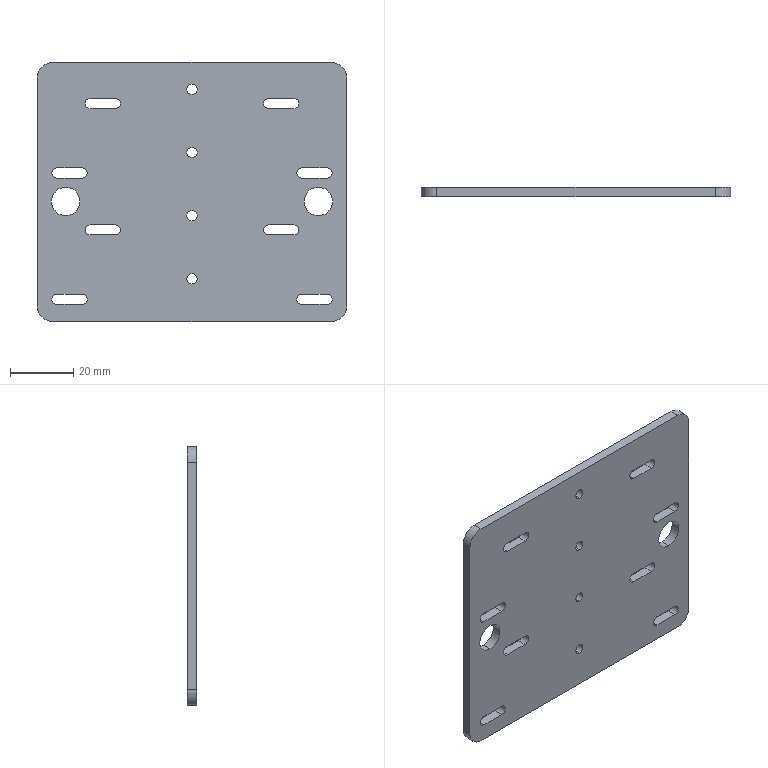Part | SolidWorks | features BaseBody 1 | 1 solid | 54 faces | box 98 x 3 x 82 mm | volume 22758 mm3 | cylinder 32 | plane 22 | commonest cylinder face diameters 3.2 x24 9 x4 10 x4